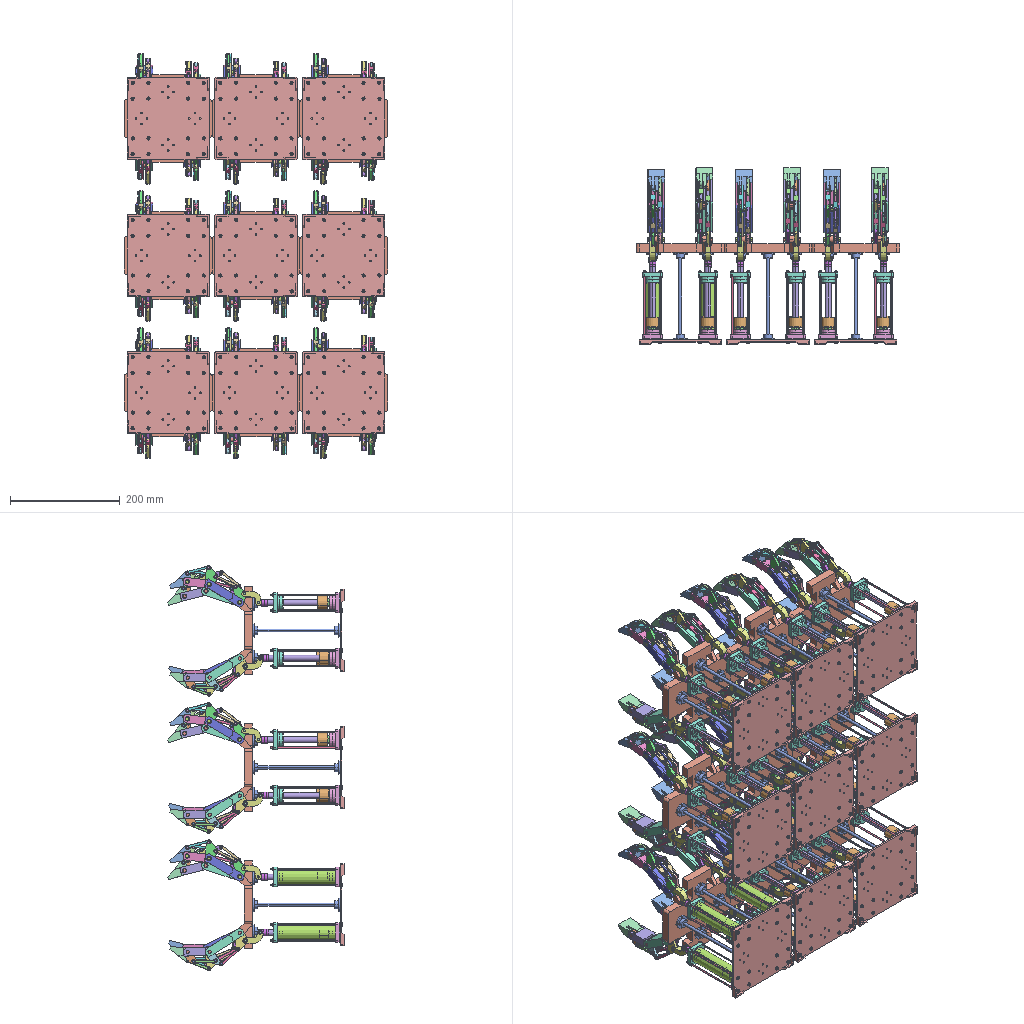Assembly | SolidWorks | 43 different items | 1929 placed | box 480 x 321 x 738 mm
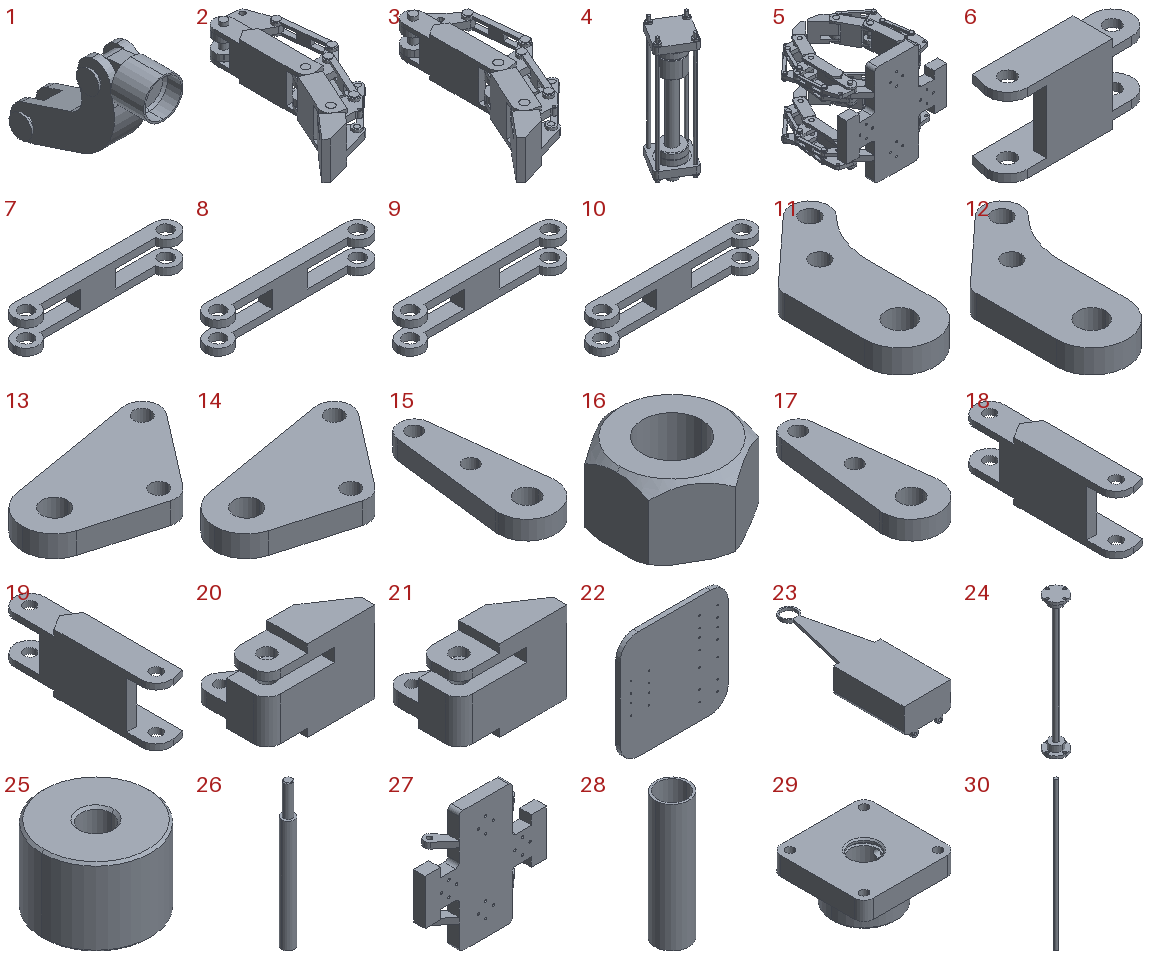Parts list (item | name | quantity | parent item | size | volume | features):
1 | (subassembly) | x36 | - | 13.3 x 41.638 x 33.297 mm | 4656 mm3 | features CompositeCurve 2
2 | (subassembly) | x18 | - | 76.237 x 131.963 x 31 mm | 53046 mm3 | features CompositeCurve 1
3 | (subassembly) | x18 | - | 75.769 x 132.444 x 31 mm | 53046 mm3 | features CompositeCurve 1
4 | (subassembly) | x36 | - | 46.813 x 46.813 x 139.8 mm | 47069 mm3 | features CompositeCurve 4
5 | (subassembly) | x1 | - | 162.597 x 146.118 x 160 mm | 452731 mm3 | -
6 | - | x18 | in 3 | 55 x 15 x 30 mm | 7665 mm3 | features ICE 3, Extrusion 1
7 | - | x36 | in 2 | 47 x 7 x 9 mm | 956.424 mm3 | features Extrusion 1, ICE 1, MirrorPattern 1
8 | - | x36 | in 3 | 47 x 7 x 9 mm | 956.424 mm3 | features Extrusion 1, ICE 1, MirrorPattern 1
9 | - | x36 | in 2 | 47 x 7 x 9 mm | 956.424 mm3 | features Extrusion 1, ICE 1, MirrorPattern 1
10 | - | x36 | in 3 | 47 x 7 x 9 mm | 956.424 mm3 | features Extrusion 1, ICE 1, MirrorPattern 1
11 | - | x18 | in 2 | 20.88 x 40 x 5 mm | 2331 mm3 | features Extrusion 1
12 | - | x18 | in 3 | 20.88 x 40 x 5 mm | 2331 mm3 | features Extrusion 1
13 | - | x36 | in 2 | 40.3 x 24.65 x 5 mm | 2970 mm3 | features Extrusion 1
14 | - | x36 | in 3 | 40.3 x 24.65 x 5 mm | 2970 mm3 | features Extrusion 1
15 | - | x18 | in 2 | 15 x 41.5 x 5 mm | 2037 mm3 | features Extrusion 1, ICE 1
16 | - | x36 | in 4 | 12.454 x 14.38 x 8 mm | 784.997 mm3 | features MBimport 1
17 | - | x18 | in 3 | 15 x 41.5 x 5 mm | 2037 mm3 | features Extrusion 1, ICE 1
18 | - | x18 | in 2 | 15 x 80 x 30 mm | 12794 mm3 | features ICE 4, Extrusion 1, Fillet 1
19 | - | x18 | in 3 | 15 x 80 x 30 mm | 12794 mm3 | features ICE 4, Extrusion 1, Fillet 1
20 | - | x18 | in 2 | 40 x 27.324 x 30 mm | 12750 mm3 | features ICE 4, Fillet 2, Extrusion 1
21 | - | x18 | in 3 | 40 x 27.324 x 30 mm | 12750 mm3 | features ICE 4, Fillet 2, Extrusion 1
22 | - | x1 | - | 120 x 5 x 120 mm | 70089 mm3 | features Extrusion 1, ICE 1
23 | - | x1 | - | 20 x 62.6 x 13.7 mm | 6966 mm3 | features ICE 2, Extrusion 1, Fillet 1
24 | - | x36 | - | 25 x 25 x 160 mm | 9208 mm3 | features ICE 1, MirrorPattern 1, Revolution 1
25 | - | x36 | in 4 | 25.2 x 25.2 x 18 mm | 8215 mm3 | features Chamfer 1, Extrusion 1
26 | - | x36 | in 4 | 10.8 x 10.8 x 124 mm | 9977 mm3 | features Chamfer 1, Extrusion 1, ICE 1
27 | - | x9 | - | 160 x 30.068 x 160 mm | 240546 mm3 | features ICE 6, Fillet 2, MirrorPattern 2, Extrusion 1
28 | - | x36 | in 4 | 28.8 x 28.8 x 108 mm | 16490 mm3 | features Extrusion 1
29 | - | x36 | in 4 | 36 x 36 x 18 mm | 12390 mm3 | features ICE 5, RevCut 3, Chamfer 2, Extrusion 1, Fillet 1
30 | - | x144 | in 4 | 2.88 x 2.88 x 131.6 mm | 857.296 mm3 | features Extrusion 1
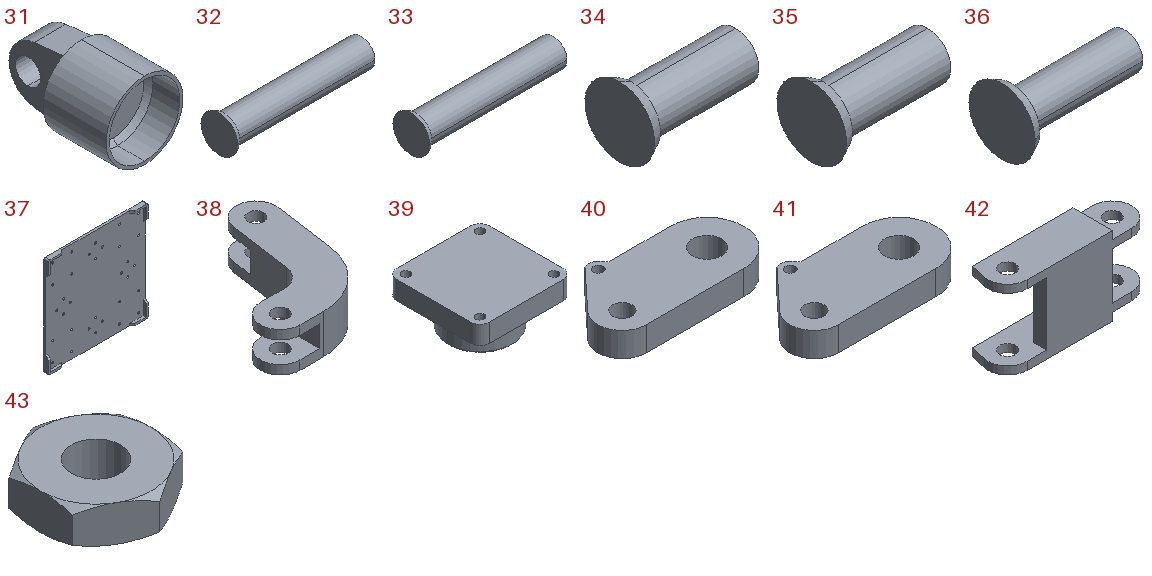31 | - | x36 | in 1 | 12.2 x 19 x 12.2 mm | 995.495 mm3 | features ICE 3, Chamfer 1, Extrusion 1
32 | - | x54 | in 2 | 31 x 8 x 8 mm | 892.474 mm3 | features Revolution 1
33 | - | x54 | in 3 | 31 x 8 x 8 mm | 892.474 mm3 | features Revolution 1
34 | - | x144 | in 2 | 10 x 6 x 6 mm | 136.921 mm3 | features Revolution 1
35 | - | x144 | in 3 | 10 x 6 x 6 mm | 136.921 mm3 | features Revolution 1
36 | - | x72 | in 1 | 13 x 7 x 7 mm | 169.342 mm3 | features Revolution 1
37 | - | x9 | - | 150 x 7 x 150 mm | 68792 mm3 | features ICE 5, Extrusion 1, Fillet 1
38 | - | x36 | in 1 | 28.109 x 34.304 x 10 mm | 3322 mm3 | features ICE 4, Extrusion 1
39 | - | x36 | in 4 | 36 x 36 x 18 mm | 11967 mm3 | features ICE 4, Chamfer 1, Extrusion 1, Fillet 1, RevCut 1
40 | - | x18 | in 2 | 32.34 x 16.75 x 5 mm | 1932 mm3 | features Extrusion 1
41 | - | x18 | in 3 | 32.34 x 16.75 x 5 mm | 1932 mm3 | features Extrusion 1
42 | - | x18 | in 2 | 55 x 15 x 30 mm | 7665 mm3 | features ICE 3, Extrusion 1
43 | - | x432 | in 4 | 5.5 x 6.351 x 1.8 mm | 38.249 mm3 | features MBimport 1
Mates (type | each side: item.copy, entity, surface, feature):
In the top assembly
Coincident | 37.1 plane | assembly plane | 3 times
Concentric | 37.1 face cylinder Cut-Extrude2 | 24.1 face cylinder Cut-Extrude4 | 2 times
Coincident | 37.1 face plane Boss-Extrude1 | 24.1 face plane Mirror1
Concentric | 37.1 face cylinder Cut-Extrude2 | 24.2 face cylinder Cut-Extrude4
Coincident | 37.1 edge | 24.2 face cylinder Cut-Extrude4
Coincident | 37.1 face plane Boss-Extrude1 | 24.2 face plane Mirror1
Concentric | 37.1 face cylinder Cut-Extrude2 | 24.3 face cylinder Cut-Extrude4 | 2 times
Coincident | 37.1 face plane Boss-Extrude1 | 24.3 face plane Mirror1
Concentric | 37.1 face cylinder Cut-Extrude2 | 24.4 face cylinder Cut-Extrude4
Coincident | 37.1 face cylinder Cut-Extrude2 | 24.4 edge
Coincident | 37.1 face plane Boss-Extrude1 | 24.4 face plane Mirror1
Concentric | 37.1 face cylinder Cut-Extrude1 | 30.1 face cylinder Boss-Extrude1
Coincident | 37.1 face plane Boss-Extrude1 | 43.1 face plane M3 nut.step<1>
Concentric | 37.1 edge | 30.2 face cylinder Boss-Extrude1
Concentric | 37.1 face cylinder Cut-Extrude1 | 30.3 face cylinder Boss-Extrude1
Concentric | 37.1 face cylinder Cut-Extrude1 | 30.4 face cylinder Boss-Extrude1
Coincident | 37.1 face plane Boss-Extrude1 | 43.2 face plane M3 nut.step<1>
Concentric | 37.1 face cylinder Cut-Extrude1 | 30.5 face cylinder Boss-Extrude1
Concentric | 37.1 face cylinder Cut-Extrude1 | 30.6 face cylinder Boss-Extrude1
Coincident | 37.1 face plane Boss-Extrude1 | 43.3 face plane M3 nut.step<1>
Concentric | 37.1 face cylinder Cut-Extrude1 | 30.7 face cylinder Boss-Extrude1
Coincident | 37.1 edge | 30.8 face cylinder Boss-Extrude1
Coincident | 37.1 face plane Boss-Extrude1 | 43.4 face plane M3 nut.step<1>
Concentric | 30.8 edge | 43.5 face cylinder M3 nut.step<1>
Coincident | 37.1 face plane Boss-Extrude1 | 43.5 face plane M3 nut.step<1>
Concentric | 30.7 face cylinder Boss-Extrude1 | 43.6 face cylinder M3 nut.step<1>
Coincident | 37.1 face plane Boss-Extrude1 | 43.6 face plane M3 nut.step<1>
Concentric | 30.9 face cylinder Boss-Extrude1 | 43.7 face cylinder M3 nut.step<1>
Concentric | 30.10 face cylinder Boss-Extrude1 | 43.8 face cylinder M3 nut.step<1>
Coincident | 37.1 face plane Boss-Extrude1 | 43.8 face plane M3 nut.step<1>
Coincident | 37.1 face plane Boss-Extrude1 | 43.7 face plane M3 nut.step<1>
Concentric | 30.6 face cylinder Boss-Extrude1 | 43.9 face cylinder M3 nut.step<1>
Concentric | 30.5 edge | 43.10 face cylinder M3 nut.step<1>
Concentric | 30.11 face cylinder Boss-Extrude1 | 43.11 face cylinder M3 nut.step<1>
Concentric | 30.12 face cylinder Boss-Extrude1 | 43.12 face cylinder M3 nut.step<1>
Coincident | 37.1 face plane Boss-Extrude1 | 43.12 face plane M3 nut.step<1>
Coincident | 37.1 face plane Boss-Extrude1 | 43.11 face plane M3 nut.step<1>
Coincident | 37.1 face plane Boss-Extrude1 | 43.10 face plane M3 nut.step<1>
Coincident | 37.1 face plane Boss-Extrude1 | 43.9 face plane M3 nut.step<1>
Concentric | 30.3 face cylinder Boss-Extrude1 | 43.13 face cylinder M3 nut.step<1>
Concentric | 30.13 face cylinder Boss-Extrude1 | 43.14 face cylinder M3 nut.step<1>
Concentric | 30.14 face cylinder Boss-Extrude1 | 43.15 face cylinder M3 nut.step<1>
Concentric | 30.4 face cylinder Boss-Extrude1 | 43.16 face cylinder M3 nut.step<1>
Coincident | 37.1 face plane Boss-Extrude1 | 43.13 face plane M3 nut.step<1>
Coincident | 37.1 face plane Boss-Extrude1 | 43.15 face plane M3 nut.step<1>
Coincident | 37.1 face plane Boss-Extrude1 | 43.14 face plane M3 nut.step<1>
Coincident | 37.1 face plane Boss-Extrude1 | 43.16 face plane M3 nut.step<1>
Concentric | 30.2 face cylinder Boss-Extrude1 | 43.17 face cylinder M3 nut.step<1>
Concentric | 30.1 face cylinder Boss-Extrude1 | 43.18 face cylinder M3 nut.step<1>
Concentric | 30.15 face cylinder Boss-Extrude1 | 43.19 face cylinder M3 nut.step<1>
Concentric | 30.16 face cylinder Boss-Extrude1 | 43.20 face cylinder M3 nut.step<1>
Coincident | 37.1 face plane Boss-Extrude1 | 43.20 edge
Coincident | 37.1 face plane Boss-Extrude1 | 43.18 face plane M3 nut.step<1>
Coincident | 37.1 face plane Boss-Extrude1 | 43.19 face plane M3 nut.step<1>
Coincident | 37.1 face plane Boss-Extrude1 | 43.17 face plane M3 nut.step<1>
Concentric | 26.1 face cylinder Boss-Extrude1 | 31.1 face cylinder Boss-Extrude1
Coincident | 26.1 face plane Boss-Extrude1 | 31.1 face plane Cut-Extrude2
Concentric | 26.2 face cylinder Boss-Extrude1 | 31.2 face cylinder Cut-Extrude2
Coincident | 26.2 face plane Boss-Extrude1 | 31.2 face plane Cut-Extrude2
Concentric | 26.3 face cylinder Boss-Extrude1 | 31.3 face cylinder Cut-Extrude2
Coincident | 26.3 face plane Boss-Extrude1 | 31.3 face plane Cut-Extrude2
Concentric | 26.4 face cylinder Boss-Extrude1 | 31.4 edge
Coincident | 26.4 face plane Boss-Extrude1 | 31.4 face plane Cut-Extrude2
Coincident | 27.1 select_type:24 | assembly select_type:10
Coincident | 24.2 face plane Revolve2 | 27.1 face plane Boss-Extrude1
Concentric | 24.1 face cylinder Cut-Extrude4 | 27.1 face cylinder Cut-Extrude4
Concentric | 27.1 face cylinder Boss-Extrude4 | 33.1 face cylinder Revolve1
Coincident | 27.1 face plane Boss-Extrude4 | 17.1 face plane Boss-Extrude1
Concentric | 27.1 face cylinder Mirror2 | 32.1 face cylinder Revolve1
Concentric | 27.1 face cylinder Mirror2 | 33.2 face cylinder Revolve1
Coincident | 27.1 face plane Mirror2 | 14.1 face plane Boss-Extrude1
Concentric | 27.1 face cylinder Mirror1 | 32.2 face cylinder Revolve1
Concentric | 36.1 face cylinder Revolve1 | 13.1 face cylinder Boss-Extrude1
Concentric | 36.2 face cylinder Revolve1 | 14.1 face cylinder Boss-Extrude1
Concentric | 36.3 face cylinder Revolve1 | 14.2 face cylinder Boss-Extrude1
Concentric | 36.4 face cylinder Revolve1 | 13.2 face cylinder Boss-Extrude1
Coincident | 38.1 face plane Cut-Extrude5 | 13.2 face plane Boss-Extrude1
Coincident | 38.2 face plane Cut-Extrude5 | 13.1 face plane Boss-Extrude1
In subassembly 4
Coincident | 28.1 plane | 4.1 plane | 3 times
Concentric | 25.1 face cylinder Boss-Extrude1 | 26.5 face cylinder Cut-Extrude1
Coincident | 25.1 face plane Boss-Extrude1 | 26.5 face plane Cut-Extrude1
Concentric | 28.1 face cylinder Boss-Extrude1 | 26.5 face cylinder Boss-Extrude1
Concentric | 26.5 face cylinder Cut-Extrude1 | 16.1 face cylinder GB/T 6186-2000 [type 2 all-metal hex lock nut, grade 9, M8].step<1>
Coincident | 25.1 face plane Boss-Extrude1 | 16.1 face plane GB/T 6186-2000 [type 2 all-metal hex lock nut, grade 9, M8].step<1>
Concentric | 28.1 face cylinder Boss-Extrude1 | 39.1 face cylinder Boss-Extrude1
Coincident | 28.1 face plane Boss-Extrude1 | 39.1 face plane Cut-Extrude1
Coincident | 29.1 edge | 26.5 face cylinder Boss-Extrude1
Coincident | 28.1 edge | 29.1 face plane Cut-Extrude1
Coincident | 39.1 face plane Boss-Extrude2 | 29.1 face plane Boss-Extrude2
Concentric | 39.1 face cylinder Cut-Extrude2 | 30.17 face cylinder Boss-Extrude1
Concentric | 39.1 face cylinder Cut-Extrude2 | 30.18 face cylinder Boss-Extrude1
Concentric | 39.1 edge | 30.19 face cylinder Boss-Extrude1
Concentric | 39.1 edge | 30.20 face cylinder Boss-Extrude1
Coincident | 30.17 face plane Boss-Extrude1 | 30.18 face plane Boss-Extrude1
Coincident | 30.17 face plane Boss-Extrude1 | 30.19 face plane Boss-Extrude1
Coincident | 30.20 face plane Boss-Extrude1 | 30.18 face plane Boss-Extrude1
Concentric | 30.19 face cylinder Boss-Extrude1 | 43.5 face cylinder M3 nut.step<1>
Concentric | 30.20 face cylinder Boss-Extrude1 | 43.6 face cylinder M3 nut.step<1>
Concentric | 30.17 face cylinder Boss-Extrude1 | 43.7 face cylinder M3 nut.step<1>
Concentric | 30.18 face cylinder Boss-Extrude1 | 43.8 face cylinder M3 nut.step<1>
Concentric | 30.17 face cylinder Boss-Extrude1 | 43.9 face cylinder M3 nut.step<1>
Concentric | 30.19 face cylinder Boss-Extrude1 | 43.11 face cylinder M3 nut.step<1>
Concentric | 30.20 face cylinder Boss-Extrude1 | 43.10 face cylinder M3 nut.step<1>
Concentric | 30.18 face cylinder Boss-Extrude1 | 43.12 face cylinder M3 nut.step<1>
Coincident | 39.1 face plane Boss-Extrude2 | 43.7 face plane M3 nut.step<1>
Coincident | 39.1 face plane Boss-Extrude2 | 43.8 face plane M3 nut.step<1>
Coincident | 39.1 face plane Boss-Extrude2 | 43.5 face plane M3 nut.step<1>
Coincident | 39.1 face plane Boss-Extrude2 | 43.6 face plane M3 nut.step<1>
Coincident | 29.1 face plane Boss-Extrude2 | 43.10 face plane M3 nut.step<1>
Coincident | 29.1 face plane Boss-Extrude2 | 43.12 face plane M3 nut.step<1>
Coincident | 29.1 face plane Boss-Extrude2 | 43.9 face plane M3 nut.step<1>
Coincident | 29.1 face plane Boss-Extrude2 | 43.11 face plane M3 nut.step<1>
LimitDistanceDim | 25.1 face plane Boss-Extrude1 | 29.1 face plane Boss-Extrude1
DistanceDim | 30.18 face plane Boss-Extrude1 | 43.8 face plane M3 nut.step<1>
In subassembly 3
Concentric | 19.1 face cylinder Boss-Extrude1 | 17.2 face cylinder Boss-Extrude1
Coincident | 19.1 face plane Cut-Extrude1 | 17.2 face plane Boss-Extrude1
Concentric | 19.1 face cylinder Boss-Extrude1 | 14.3 face cylinder Boss-Extrude1
Coincident | 19.1 face plane Cut-Extrude1 | 14.3 face plane Boss-Extrude1
Coincident | 10.1 edge | 14.3 face cylinder Boss-Extrude1
Coincident | 10.1 face plane Mirror1 | 14.3 face plane Boss-Extrude1
Concentric | 19.1 face cylinder Boss-Extrude1 | 14.4 face cylinder Boss-Extrude1
Concentric | 19.1 face cylinder Boss-Extrude1 | 6.1 face cylinder Boss-Extrude1
Coincident | 19.1 face plane Cut-Extrude1 | 6.1 face plane Cut-Extrude1
Coincident | 6.1 face plane Cut-Extrude2 | 14.4 face plane Boss-Extrude1
Concentric | 10.1 face cylinder Boss-Extrude1 | 14.4 face cylinder Boss-Extrude1
Concentric | 19.1 face cylinder Boss-Extrude1 | 12.1 face cylinder Boss-Extrude1
Coincident | 6.1 face plane Cut-Extrude2 | 12.1 face plane Boss-Extrude1
Concentric | 12.1 face cylinder Boss-Extrude1 | 10.2 face cylinder Boss-Extrude1
Coincident | 12.1 face plane Boss-Extrude1 | 10.2 face plane Cut-Extrude1
Concentric | 17.2 face cylinder Boss-Extrude1 | 10.2 face cylinder Boss-Extrude1
Concentric | 8.1 face cylinder Boss-Extrude1 | 14.4 face cylinder Boss-Extrude1
Coincident | 8.1 face plane Cut-Extrude1 | 14.4 face plane Boss-Extrude1
Concentric | 6.1 face cylinder Boss-Extrude1 | 21.1 face cylinder Cut-Extrude3
Coincident | 6.1 face plane Cut-Extrude1 | 21.1 face plane Cut-Extrude1
Concentric | 41.1 face cylinder Boss-Extrude1 | 6.1 face cylinder Boss-Extrude1
Coincident | 41.1 face plane Boss-Extrude1 | 21.1 face plane Cut-Extrude2
Concentric | 8.1 face cylinder Boss-Extrude1 | 21.1 face cylinder Boss-Extrude3
Concentric | 12.1 face cylinder Boss-Extrude1 | 8.2 face cylinder Boss-Extrude1
Coincident | 12.1 face plane Boss-Extrude1 | 8.2 face plane Cut-Extrude1
Concentric | 41.1 face cylinder Boss-Extrude1 | 8.2 face cylinder Boss-Extrude1
Concentric | 6.1 face cylinder Boss-Extrude1 | 33.3 face cylinder Revolve1
Coincident | 6.1 face plane Boss-Extrude1 | 33.3 face plane Revolve1
Concentric | 8.1 face cylinder Boss-Extrude1 | 35.1 face cylinder Revolve1
Coincident | 8.1 face plane Boss-Extrude1 | 35.1 face plane Revolve1
Concentric | 8.2 face cylinder Boss-Extrude1 | 35.2 face cylinder Revolve1
Coincident | 8.2 face plane Boss-Extrude1 | 35.2 face plane Revolve1
Concentric | 8.1 face cylinder Boss-Extrude1 | 35.3 face cylinder Revolve1
Coincident | 8.1 face plane Boss-Extrude1 | 35.3 face plane Revolve1
Concentric | 8.2 face cylinder Boss-Extrude1 | 35.4 face cylinder Revolve1
Coincident | 8.2 face plane Boss-Extrude1 | 35.4 face plane Revolve1
Concentric | 10.2 face cylinder Boss-Extrude1 | 35.5 face cylinder Revolve1
Coincident | 10.2 face plane Boss-Extrude1 | 35.5 face plane Revolve1
Concentric | 10.1 face cylinder Boss-Extrude1 | 35.6 face cylinder Revolve1
Coincident | 10.1 face plane Boss-Extrude1 | 35.6 face plane Revolve1
Concentric | 10.2 face cylinder Boss-Extrude1 | 35.7 face cylinder Revolve1
Coincident | 10.2 face plane Boss-Extrude1 | 35.7 face plane Revolve1
Concentric | 10.1 face cylinder Boss-Extrude1 | 35.8 face cylinder Revolve1
Coincident | 10.1 face plane Boss-Extrude1 | 35.8 face plane Revolve1
Concentric | 19.1 face cylinder Boss-Extrude1 | 33.4 face cylinder Revolve1
Coincident | 19.1 face plane Boss-Extrude1 | 33.4 face plane Revolve1
Concentric | 19.1 face cylinder Boss-Extrude1 | 33.5 face cylinder Revolve1
Coincident | 19.1 face plane Boss-Extrude1 | 33.5 face plane Revolve1
In subassembly 1
Coincident | 31.5 plane | 1.1 plane | 3 times
Concentric | 38.3 edge | 31.5 face cylinder Cut-Extrude1
Coincident | 38.3 face plane Cut-Extrude2 | 31.5 face plane Boss-Extrude2
Concentric | 38.3 edge | 36.5 face cylinder Revolve1
DistanceDim | 36.5 face plane Revolve1 | 38.3 face plane Boss-Extrude1
Concentric | 38.3 face cylinder Cut-Extrude3 | 36.6 face cylinder Revolve1
DistanceDim | 36.6 face plane Revolve1 | 38.3 face plane Boss-Extrude1
In subassembly 2
Concentric | 18.1 face cylinder Boss-Extrude1 | 13.3 face cylinder Boss-Extrude1
Concentric | 18.1 face cylinder Boss-Extrude1 | 42.1 face cylinder Boss-Extrude1
Coincident | 18.1 face plane Cut-Extrude1 | 42.1 face plane Cut-Extrude1
Coincident | 42.1 face plane Cut-Extrude2 | 13.3 face plane Boss-Extrude1
Concentric | 9.1 face cylinder Boss-Extrude1 | 13.3 face cylinder Boss-Extrude1
Concentric | 18.1 face cylinder Boss-Extrude1 | 11.1 face cylinder Boss-Extrude1
Coincident | 42.1 face plane Cut-Extrude2 | 11.1 face plane Boss-Extrude1
Concentric | 11.1 face cylinder Boss-Extrude1 | 9.2 face cylinder Boss-Extrude1
Coincident | 11.1 face plane Boss-Extrude1 | 9.2 face plane Cut-Extrude1
Concentric | 7.1 face cylinder Boss-Extrude1 | 13.3 face cylinder Boss-Extrude1
Coincident | 7.1 face plane Cut-Extrude1 | 13.3 face plane Boss-Extrude1
Concentric | 42.1 face cylinder Boss-Extrude1 | 20.1 face cylinder Cut-Extrude3
Coincident | 42.1 face plane Cut-Extrude1 | 20.1 face plane Cut-Extrude1
Concentric | 40.1 face cylinder Boss-Extrude1 | 42.1 face cylinder Boss-Extrude1
Coincident | 40.1 face plane Boss-Extrude1 | 20.1 face plane Cut-Extrude2
Concentric | 7.1 face cylinder Boss-Extrude1 | 20.1 face cylinder Boss-Extrude3
Concentric | 11.1 face cylinder Boss-Extrude1 | 7.2 face cylinder Boss-Extrude1
Coincident | 11.1 face plane Boss-Extrude1 | 7.2 face plane Cut-Extrude1
Concentric | 40.1 face cylinder Boss-Extrude1 | 7.2 face cylinder Boss-Extrude1
Concentric | 42.1 face cylinder Boss-Extrude1 | 32.3 face cylinder Revolve1
Coincident | 42.1 face plane Boss-Extrude1 | 32.3 face plane Revolve1
Concentric | 7.1 face cylinder Boss-Extrude1 | 34.1 face cylinder Revolve1
Coincident | 7.1 face plane Boss-Extrude1 | 34.1 face plane Revolve1
Concentric | 7.2 face cylinder Boss-Extrude1 | 34.2 face cylinder Revolve1
Coincident | 7.2 face plane Boss-Extrude1 | 34.2 face plane Revolve1
Concentric | 7.1 face cylinder Boss-Extrude1 | 34.3 face cylinder Revolve1
Coincident | 7.1 face plane Boss-Extrude1 | 34.3 face plane Revolve1
Concentric | 7.2 face cylinder Boss-Extrude1 | 34.4 face cylinder Revolve1
Coincident | 7.2 face plane Boss-Extrude1 | 34.4 face plane Revolve1
Concentric | 9.2 face cylinder Boss-Extrude1 | 34.5 face cylinder Revolve1
Coincident | 9.2 face plane Boss-Extrude1 | 34.5 face plane Revolve1
Concentric | 9.1 face cylinder Boss-Extrude1 | 34.6 face cylinder Revolve1
Coincident | 9.1 face plane Boss-Extrude1 | 34.6 face plane Revolve1
Concentric | 9.2 face cylinder Boss-Extrude1 | 34.7 face cylinder Revolve1
Coincident | 9.2 face plane Boss-Extrude1 | 34.7 face plane Revolve1
Concentric | 9.1 face cylinder Boss-Extrude1 | 34.8 face cylinder Revolve1
Coincident | 9.1 face plane Boss-Extrude1 | 34.8 face plane Revolve1
Concentric | 18.1 face cylinder Boss-Extrude1 | 32.4 face cylinder Revolve1
Coincident | 18.1 face plane Boss-Extrude1 | 32.4 face plane Revolve1
Concentric | 18.1 face cylinder Boss-Extrude1 | 32.5 face cylinder Revolve1
Coincident | 18.1 face plane Boss-Extrude1 | 32.5 face plane Revolve1
Concentric | 15.1 face cylinder Boss-Extrude1 | 34.8 face cylinder Revolve1
Concentric | 15.1 face cylinder Boss-Extrude1 | 32.5 face cylinder Revolve1
Coincident | 9.1 face plane Mirror1 | 15.1 face plane Boss-Extrude1
Concentric | 13.4 face cylinder Boss-Extrude1 | 34.7 face cylinder Revolve1
Concentric | 13.4 edge | 32.5 face cylinder Revolve1
Coincident | 13.4 face plane Boss-Extrude1 | 9.2 face plane Mirror1